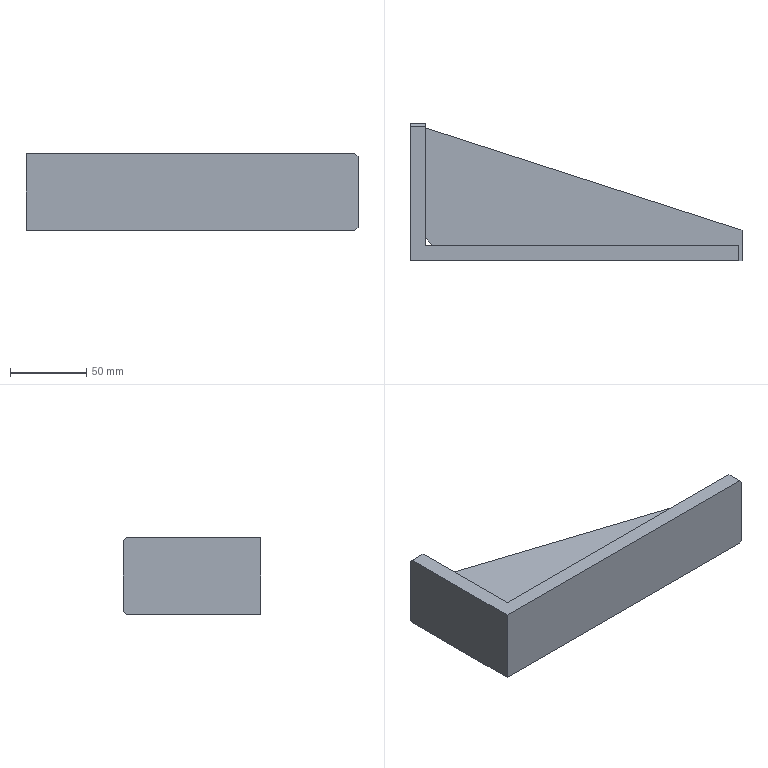Part | SolidWorks | features Chamfer 1, Extrusion 1, ICE 1 | 1 solid | 16 faces | box 217.5 x 90 x 50 mm | volume 220780 mm3 | plane 16
STEP:
#1=CARTESIAN_POINT('',(0.,88.,25.));
#2=VERTEX_POINT('',#1);
#3=CARTESIAN_POINT('',(0.,0.,25.));
#4=VERTEX_POINT('',#3);
#5=CARTESIAN_POINT('',(0.,90.,25.));
#6=DIRECTION('',(0.,-1.,0.));
#7=VECTOR('',#6,1000.);
#8=LINE('',#5,#7);
#9=EDGE_CURVE('',#2,#4,#8,.T.);
#10=ORIENTED_EDGE('',*,*,#9,.F.);
#11=CARTESIAN_POINT('',(0.,90.,23.));
#12=VERTEX_POINT('',#11);
#13=CARTESIAN_POINT('',(0.,88.,25.));
#14=DIRECTION('',(0.,0.7071,-0.7071));
#15=VECTOR('',#14,1000.);
#16=LINE('',#13,#15);
#17=EDGE_CURVE('',#2,#12,#16,.T.);
#18=ORIENTED_EDGE('',*,*,#17,.T.);
#19=CARTESIAN_POINT('',(0.,90.,-23.));
#20=VERTEX_POINT('',#19);
#21=CARTESIAN_POINT('',(0.,90.,25.));
#22=DIRECTION('',(0.,0.,-1.));
#23=VECTOR('',#22,1000.);
#24=LINE('',#21,#23);
#25=EDGE_CURVE('',#12,#20,#24,.T.);
#26=ORIENTED_EDGE('',*,*,#25,.T.);
#27=CARTESIAN_POINT('',(0.,88.,-25.));
#28=VERTEX_POINT('',#27);
#29=CARTESIAN_POINT('',(0.,90.,-23.));
#30=DIRECTION('',(0.,-0.7071,-0.7071));
#31=VECTOR('',#30,1000.);
#32=LINE('',#29,#31);
#33=EDGE_CURVE('',#20,#28,#32,.T.);
#34=ORIENTED_EDGE('',*,*,#33,.T.);
#35=CARTESIAN_POINT('',(0.,0.,-25.));
#36=VERTEX_POINT('',#35);
#37=CARTESIAN_POINT('',(0.,90.,-25.));
#38=DIRECTION('',(0.,-1.,0.));
#39=VECTOR('',#38,1000.);
#40=LINE('',#37,#39);
#41=EDGE_CURVE('',#28,#36,#40,.T.);
#42=ORIENTED_EDGE('',*,*,#41,.T.);
#43=CARTESIAN_POINT('',(0.,0.,25.));
#44=DIRECTION('',(0.,0.,-1.));
#45=VECTOR('',#44,1000.);
#46=LINE('',#43,#45);
#47=EDGE_CURVE('',#4,#36,#46,.T.);
#48=ORIENTED_EDGE('',*,*,#47,.F.);
#49=EDGE_LOOP('',(#10,#18,#26,#34,#42,#48));
#50=FACE_OUTER_BOUND('',#49,.T.);
#51=CARTESIAN_POINT('',(0.,90.,25.));
#52=DIRECTION('',(1.,0.,0.));
#53=DIRECTION('',(0.,1.,0.));
#54=AXIS2_PLACEMENT_3D('',#51,#52,#53);
#55=PLANE('',#54);
#56=ADVANCED_FACE('',(#50),#55,.F.);
#57=CARTESIAN_POINT('',(215.5,0.,-25.));
#58=VERTEX_POINT('',#57);
#59=CARTESIAN_POINT('',(0.,0.,-25.));
#60=DIRECTION('',(1.,0.,0.));
#61=VECTOR('',#60,1000.);
#62=LINE('',#59,#61);
#63=EDGE_CURVE('',#36,#58,#62,.T.);
#64=ORIENTED_EDGE('',*,*,#63,.T.);
#65=CARTESIAN_POINT('',(217.5,0.,-23.));
#66=VERTEX_POINT('',#65);
#67=CARTESIAN_POINT('',(217.5,0.,-23.));
#68=DIRECTION('',(0.7071,0.,0.7071));
#69=VECTOR('',#68,1000.);
#70=LINE('',#67,#69);
#71=EDGE_CURVE('',#58,#66,#70,.T.);
#72=ORIENTED_EDGE('',*,*,#71,.T.);
#73=CARTESIAN_POINT('',(217.5,0.,23.));
#74=VERTEX_POINT('',#73);
#75=CARTESIAN_POINT('',(217.5,0.,25.));
#76=DIRECTION('',(0.,0.,-1.));
#77=VECTOR('',#76,1000.);
#78=LINE('',#75,#77);
#79=EDGE_CURVE('',#74,#66,#78,.T.);
#80=ORIENTED_EDGE('',*,*,#79,.F.);
#81=CARTESIAN_POINT('',(215.5,0.,25.));
#82=VERTEX_POINT('',#81);
#83=CARTESIAN_POINT('',(215.5,0.,25.));
#84=DIRECTION('',(-0.7071,0.,0.7071));
#85=VECTOR('',#84,1000.);
#86=LINE('',#83,#85);
#87=EDGE_CURVE('',#74,#82,#86,.T.);
#88=ORIENTED_EDGE('',*,*,#87,.T.);
#89=CARTESIAN_POINT('',(0.,0.,25.));
#90=DIRECTION('',(1.,0.,0.));
#91=VECTOR('',#90,1000.);
#92=LINE('',#89,#91);
#93=EDGE_CURVE('',#4,#82,#92,.T.);
#94=ORIENTED_EDGE('',*,*,#93,.F.);
#95=ORIENTED_EDGE('',*,*,#47,.T.);
#96=EDGE_LOOP('',(#64,#72,#80,#88,#94,#95));
#97=FACE_OUTER_BOUND('',#96,.T.);
#98=CARTESIAN_POINT('',(0.,0.,25.));
#99=DIRECTION('',(0.,1.,0.));
#100=DIRECTION('',(0.,0.,1.));
#101=AXIS2_PLACEMENT_3D('',#98,#99,#100);
#102=PLANE('',#101);
#103=ADVANCED_FACE('',(#97),#102,.F.);
#104=ORIENTED_EDGE('',*,*,#79,.T.);
#105=CARTESIAN_POINT('',(217.5,10.,-23.));
#106=VERTEX_POINT('',#105);
#107=CARTESIAN_POINT('',(217.5,0.,-23.));
#108=DIRECTION('',(0.,1.,0.));
#109=VECTOR('',#108,1000.);
#110=LINE('',#107,#109);
#111=EDGE_CURVE('',#66,#106,#110,.T.);
#112=ORIENTED_EDGE('',*,*,#111,.T.);
#113=CARTESIAN_POINT('',(217.5,10.,-4.));
#114=VERTEX_POINT('',#113);
#115=CARTESIAN_POINT('',(217.5,10.,25.));
#116=DIRECTION('',(0.,0.,-1.));
#117=VECTOR('',#116,1000.);
#118=LINE('',#115,#117);
#119=EDGE_CURVE('',#114,#106,#118,.T.);
#120=ORIENTED_EDGE('',*,*,#119,.F.);
#121=CARTESIAN_POINT('',(217.5,20.,-4.));
#122=VERTEX_POINT('',#121);
#123=CARTESIAN_POINT('',(217.5,20.,-4.));
#124=DIRECTION('',(0.,1.,0.));
#125=VECTOR('',#124,1000.);
#126=LINE('',#123,#125);
#127=EDGE_CURVE('',#114,#122,#126,.T.);
#128=ORIENTED_EDGE('',*,*,#127,.T.);
#129=CARTESIAN_POINT('',(217.5,20.,4.));
#130=VERTEX_POINT('',#129);
#131=CARTESIAN_POINT('',(217.5,20.,4.));
#132=DIRECTION('',(0.,0.,-1.));
#133=VECTOR('',#132,1000.);
#134=LINE('',#131,#133);
#135=EDGE_CURVE('',#130,#122,#134,.T.);
#136=ORIENTED_EDGE('',*,*,#135,.F.);
#137=CARTESIAN_POINT('',(217.5,10.,4.));
#138=VERTEX_POINT('',#137);
#139=CARTESIAN_POINT('',(217.5,20.,4.));
#140=DIRECTION('',(0.,1.,0.));
#141=VECTOR('',#140,1000.);
#142=LINE('',#139,#141);
#143=EDGE_CURVE('',#138,#130,#142,.T.);
#144=ORIENTED_EDGE('',*,*,#143,.F.);
#145=CARTESIAN_POINT('',(217.5,10.,23.));
#146=VERTEX_POINT('',#145);
#147=CARTESIAN_POINT('',(217.5,10.,25.));
#148=DIRECTION('',(0.,0.,-1.));
#149=VECTOR('',#148,1000.);
#150=LINE('',#147,#149);
#151=EDGE_CURVE('',#146,#138,#150,.T.);
#152=ORIENTED_EDGE('',*,*,#151,.F.);
#153=CARTESIAN_POINT('',(217.5,0.,23.));
#154=DIRECTION('',(0.,-1.,0.));
#155=VECTOR('',#154,1000.);
#156=LINE('',#153,#155);
#157=EDGE_CURVE('',#146,#74,#156,.T.);
#158=ORIENTED_EDGE('',*,*,#157,.T.);
#159=EDGE_LOOP('',(#104,#112,#120,#128,#136,#144,#152,#158));
#160=FACE_OUTER_BOUND('',#159,.T.);
#161=CARTESIAN_POINT('',(217.5,0.,25.));
#162=DIRECTION('',(-1.,0.,0.));
#163=DIRECTION('',(0.,0.,1.));
#164=AXIS2_PLACEMENT_3D('',#161,#162,#163);
#165=PLANE('',#164);
#166=ADVANCED_FACE('',(#160),#165,.F.);
#167=ORIENTED_EDGE('',*,*,#119,.T.);
#168=CARTESIAN_POINT('',(215.5,10.,-25.));
#169=VERTEX_POINT('',#168);
#170=CARTESIAN_POINT('',(217.5,10.,-23.));
#171=DIRECTION('',(-0.7071,0.,-0.7071));
#172=VECTOR('',#171,1000.);
#173=LINE('',#170,#172);
#174=EDGE_CURVE('',#106,#169,#173,.T.);
#175=ORIENTED_EDGE('',*,*,#174,.T.);
#176=CARTESIAN_POINT('',(10.,10.,-25.));
#177=VERTEX_POINT('',#176);
#178=CARTESIAN_POINT('',(217.5,10.,-25.));
#179=DIRECTION('',(-1.,0.,0.));
#180=VECTOR('',#179,1000.);
#181=LINE('',#178,#180);
#182=EDGE_CURVE('',#169,#177,#181,.T.);
#183=ORIENTED_EDGE('',*,*,#182,.T.);
#184=CARTESIAN_POINT('',(10.,10.,25.));
#185=VERTEX_POINT('',#184);
#186=CARTESIAN_POINT('',(10.,10.,25.));
#187=DIRECTION('',(0.,0.,-1.));
#188=VECTOR('',#187,1000.);
#189=LINE('',#186,#188);
#190=EDGE_CURVE('',#185,#177,#189,.T.);
#191=ORIENTED_EDGE('',*,*,#190,.F.);
#192=CARTESIAN_POINT('',(215.5,10.,25.));
#193=VERTEX_POINT('',#192);
#194=CARTESIAN_POINT('',(217.5,10.,25.));
#195=DIRECTION('',(-1.,0.,0.));
#196=VECTOR('',#195,1000.);
#197=LINE('',#194,#196);
#198=EDGE_CURVE('',#193,#185,#197,.T.);
#199=ORIENTED_EDGE('',*,*,#198,.F.);
#200=CARTESIAN_POINT('',(215.5,10.,25.));
#201=DIRECTION('',(0.7071,0.,-0.7071));
#202=VECTOR('',#201,1000.);
#203=LINE('',#200,#202);
#204=EDGE_CURVE('',#193,#146,#203,.T.);
#205=ORIENTED_EDGE('',*,*,#204,.T.);
#206=ORIENTED_EDGE('',*,*,#151,.T.);
#207=CARTESIAN_POINT('',(15.,10.,4.));
#208=VERTEX_POINT('',#207);
#209=CARTESIAN_POINT('',(217.5,10.,4.));
#210=DIRECTION('',(1.,0.,0.));
#211=VECTOR('',#210,1000.);
#212=LINE('',#209,#211);
#213=EDGE_CURVE('',#208,#138,#212,.T.);
#214=ORIENTED_EDGE('',*,*,#213,.F.);
#215=CARTESIAN_POINT('',(15.,10.,-4.));
#216=VERTEX_POINT('',#215);
#217=CARTESIAN_POINT('',(15.,10.,4.));
#218=DIRECTION('',(0.,0.,-1.));
#219=VECTOR('',#218,1000.);
#220=LINE('',#217,#219);
#221=EDGE_CURVE('',#208,#216,#220,.T.);
#222=ORIENTED_EDGE('',*,*,#221,.T.);
#223=CARTESIAN_POINT('',(217.5,10.,-4.));
#224=DIRECTION('',(1.,0.,0.));
#225=VECTOR('',#224,1000.);
#226=LINE('',#223,#225);
#227=EDGE_CURVE('',#216,#114,#226,.T.);
#228=ORIENTED_EDGE('',*,*,#227,.T.);
#229=EDGE_LOOP('',(#167,#175,#183,#191,#199,#205,#206,#214,#222,#228));
#230=FACE_OUTER_BOUND('',#229,.T.);
#231=CARTESIAN_POINT('',(217.5,10.,25.));
#232=DIRECTION('',(0.,-1.,0.));
#233=DIRECTION('',(1.,0.,0.));
#234=AXIS2_PLACEMENT_3D('',#231,#232,#233);
#235=PLANE('',#234);
#236=ADVANCED_FACE('',(#230),#235,.F.);
#237=CARTESIAN_POINT('',(10.,15.,4.));
#238=VERTEX_POINT('',#237);
#239=CARTESIAN_POINT('',(10.,15.,-4.));
#240=VERTEX_POINT('',#239);
#241=CARTESIAN_POINT('',(10.,15.,4.));
#242=DIRECTION('',(0.,0.,-1.));
#243=VECTOR('',#242,1000.);
#244=LINE('',#241,#243);
#245=EDGE_CURVE('',#238,#240,#244,.T.);
#246=ORIENTED_EDGE('',*,*,#245,.F.);
#247=CARTESIAN_POINT('',(10.,87.,4.));
#248=VERTEX_POINT('',#247);
#249=CARTESIAN_POINT('',(10.,15.,4.));
#250=DIRECTION('',(0.,-1.,0.));
#251=VECTOR('',#250,1000.);
#252=LINE('',#249,#251);
#253=EDGE_CURVE('',#248,#238,#252,.T.);
#254=ORIENTED_EDGE('',*,*,#253,.F.);
#255=CARTESIAN_POINT('',(10.,87.,-4.));
#256=VERTEX_POINT('',#255);
#257=CARTESIAN_POINT('',(10.,87.,4.));
#258=DIRECTION('',(0.,0.,-1.));
#259=VECTOR('',#258,1000.);
#260=LINE('',#257,#259);
#261=EDGE_CURVE('',#248,#256,#260,.T.);
#262=ORIENTED_EDGE('',*,*,#261,.T.);
#263=CARTESIAN_POINT('',(10.,15.,-4.));
#264=DIRECTION('',(0.,-1.,0.));
#265=VECTOR('',#264,1000.);
#266=LINE('',#263,#265);
#267=EDGE_CURVE('',#256,#240,#266,.T.);
#268=ORIENTED_EDGE('',*,*,#267,.T.);
#269=EDGE_LOOP('',(#246,#254,#262,#268));
#270=FACE_BOUND('',#269,.T.);
#271=CARTESIAN_POINT('',(10.,90.,23.));
#272=VERTEX_POINT('',#271);
#273=CARTESIAN_POINT('',(10.,90.,-23.));
#274=VERTEX_POINT('',#273);
#275=CARTESIAN_POINT('',(10.,90.,25.));
#276=DIRECTION('',(0.,0.,-1.));
#277=VECTOR('',#276,1000.);
#278=LINE('',#275,#277);
#279=EDGE_CURVE('',#272,#274,#278,.T.);
#280=ORIENTED_EDGE('',*,*,#279,.F.);
#281=CARTESIAN_POINT('',(10.,88.,25.));
#282=VERTEX_POINT('',#281);
#283=CARTESIAN_POINT('',(10.,88.,25.));
#284=DIRECTION('',(0.,-0.7071,0.7071));
#285=VECTOR('',#284,1000.);
#286=LINE('',#283,#285);
#287=EDGE_CURVE('',#272,#282,#286,.T.);
#288=ORIENTED_EDGE('',*,*,#287,.T.);
#289=CARTESIAN_POINT('',(10.,10.,25.));
#290=DIRECTION('',(0.,1.,0.));
#291=VECTOR('',#290,1000.);
#292=LINE('',#289,#291);
#293=EDGE_CURVE('',#185,#282,#292,.T.);
#294=ORIENTED_EDGE('',*,*,#293,.F.);
#295=ORIENTED_EDGE('',*,*,#190,.T.);
#296=CARTESIAN_POINT('',(10.,88.,-25.));
#297=VERTEX_POINT('',#296);
#298=CARTESIAN_POINT('',(10.,10.,-25.));
#299=DIRECTION('',(0.,1.,0.));
#300=VECTOR('',#299,1000.);
#301=LINE('',#298,#300);
#302=EDGE_CURVE('',#177,#297,#301,.T.);
#303=ORIENTED_EDGE('',*,*,#302,.T.);
#304=CARTESIAN_POINT('',(10.,90.,-23.));
#305=DIRECTION('',(0.,0.7071,0.7071));
#306=VECTOR('',#305,1000.);
#307=LINE('',#304,#306);
#308=EDGE_CURVE('',#297,#274,#307,.T.);
#309=ORIENTED_EDGE('',*,*,#308,.T.);
#310=EDGE_LOOP('',(#280,#288,#294,#295,#303,#309));
#311=FACE_OUTER_BOUND('',#310,.T.);
#312=CARTESIAN_POINT('',(10.,10.,25.));
#313=DIRECTION('',(-1.,0.,0.));
#314=DIRECTION('',(0.,-1.,0.));
#315=AXIS2_PLACEMENT_3D('',#312,#313,#314);
#316=PLANE('',#315);
#317=ADVANCED_FACE('',(#270,#311),#316,.F.);
#318=ORIENTED_EDGE('',*,*,#25,.F.);
#319=CARTESIAN_POINT('',(10.,90.,23.));
#320=DIRECTION('',(1.,0.,0.));
#321=VECTOR('',#320,1000.);
#322=LINE('',#319,#321);
#323=EDGE_CURVE('',#12,#272,#322,.T.);
#324=ORIENTED_EDGE('',*,*,#323,.T.);
#325=ORIENTED_EDGE('',*,*,#279,.T.);
#326=CARTESIAN_POINT('',(10.,90.,-23.));
#327=DIRECTION('',(-1.,0.,0.));
#328=VECTOR('',#327,1000.);
#329=LINE('',#326,#328);
#330=EDGE_CURVE('',#274,#20,#329,.T.);
#331=ORIENTED_EDGE('',*,*,#330,.T.);
#332=EDGE_LOOP('',(#318,#324,#325,#331));
#333=FACE_OUTER_BOUND('',#332,.T.);
#334=CARTESIAN_POINT('',(10.,90.,25.));
#335=DIRECTION('',(0.,-1.,0.));
#336=DIRECTION('',(0.,0.,-1.));
#337=AXIS2_PLACEMENT_3D('',#334,#335,#336);
#338=PLANE('',#337);
#339=ADVANCED_FACE('',(#333),#338,.F.);
#340=ORIENTED_EDGE('',*,*,#93,.T.);
#341=CARTESIAN_POINT('',(215.5,10.,25.));
#342=DIRECTION('',(0.,1.,0.));
#343=VECTOR('',#342,1000.);
#344=LINE('',#341,#343);
#345=EDGE_CURVE('',#82,#193,#344,.T.);
#346=ORIENTED_EDGE('',*,*,#345,.T.);
#347=ORIENTED_EDGE('',*,*,#198,.T.);
#348=ORIENTED_EDGE('',*,*,#293,.T.);
#349=CARTESIAN_POINT('',(0.,88.,25.));
#350=DIRECTION('',(-1.,0.,0.));
#351=VECTOR('',#350,1000.);
#352=LINE('',#349,#351);
#353=EDGE_CURVE('',#282,#2,#352,.T.);
#354=ORIENTED_EDGE('',*,*,#353,.T.);
#355=ORIENTED_EDGE('',*,*,#9,.T.);
#356=EDGE_LOOP('',(#340,#346,#347,#348,#354,#355));
#357=FACE_OUTER_BOUND('',#356,.T.);
#358=CARTESIAN_POINT('',(0.,0.,25.));
#359=DIRECTION('',(0.,0.,1.));
#360=DIRECTION('',(1.,0.,0.));
#361=AXIS2_PLACEMENT_3D('',#358,#359,#360);
#362=PLANE('',#361);
#363=ADVANCED_FACE('',(#357),#362,.T.);
#364=ORIENTED_EDGE('',*,*,#182,.F.);
#365=CARTESIAN_POINT('',(215.5,0.,-25.));
#366=DIRECTION('',(0.,-1.,0.));
#367=VECTOR('',#366,1000.);
#368=LINE('',#365,#367);
#369=EDGE_CURVE('',#169,#58,#368,.T.);
#370=ORIENTED_EDGE('',*,*,#369,.T.);
#371=ORIENTED_EDGE('',*,*,#63,.F.);
#372=ORIENTED_EDGE('',*,*,#41,.F.);
#373=CARTESIAN_POINT('',(0.,88.,-25.));
#374=DIRECTION('',(1.,0.,0.));
#375=VECTOR('',#374,1000.);
#376=LINE('',#373,#375);
#377=EDGE_CURVE('',#28,#297,#376,.T.);
#378=ORIENTED_EDGE('',*,*,#377,.T.);
#379=ORIENTED_EDGE('',*,*,#302,.F.);
#380=EDGE_LOOP('',(#364,#370,#371,#372,#378,#379));
#381=FACE_OUTER_BOUND('',#380,.T.);
#382=CARTESIAN_POINT('',(0.,0.,-25.));
#383=DIRECTION('',(0.,0.,1.));
#384=DIRECTION('',(1.,0.,0.));
#385=AXIS2_PLACEMENT_3D('',#382,#383,#384);
#386=PLANE('',#385);
#387=ADVANCED_FACE('',(#381),#386,.F.);
#388=CARTESIAN_POINT('',(15.,10.,-4.));
#389=DIRECTION('',(0.7071,-0.7071,0.));
#390=VECTOR('',#389,1000.);
#391=LINE('',#388,#390);
#392=EDGE_CURVE('',#240,#216,#391,.T.);
#393=ORIENTED_EDGE('',*,*,#392,.T.);
#394=ORIENTED_EDGE('',*,*,#221,.F.);
#395=CARTESIAN_POINT('',(15.,10.,4.));
#396=DIRECTION('',(0.7071,-0.7071,0.));
#397=VECTOR('',#396,1000.);
#398=LINE('',#395,#397);
#399=EDGE_CURVE('',#238,#208,#398,.T.);
#400=ORIENTED_EDGE('',*,*,#399,.F.);
#401=ORIENTED_EDGE('',*,*,#245,.T.);
#402=EDGE_LOOP('',(#393,#394,#400,#401));
#403=FACE_OUTER_BOUND('',#402,.T.);
#404=CARTESIAN_POINT('',(15.,10.,4.));
#405=DIRECTION('',(0.7071,0.7071,0.));
#406=DIRECTION('',(-0.7071,0.7071,0.));
#407=AXIS2_PLACEMENT_3D('',#404,#405,#406);
#408=PLANE('',#407);
#409=ADVANCED_FACE('',(#403),#408,.F.);
#410=CARTESIAN_POINT('',(10.,87.,-4.));
#411=DIRECTION('',(-0.9516,0.3073,0.));
#412=VECTOR('',#411,1000.);
#413=LINE('',#410,#412);
#414=EDGE_CURVE('',#122,#256,#413,.T.);
#415=ORIENTED_EDGE('',*,*,#414,.T.);
#416=ORIENTED_EDGE('',*,*,#261,.F.);
#417=CARTESIAN_POINT('',(10.,87.,4.));
#418=DIRECTION('',(-0.9516,0.3073,0.));
#419=VECTOR('',#418,1000.);
#420=LINE('',#417,#419);
#421=EDGE_CURVE('',#130,#248,#420,.T.);
#422=ORIENTED_EDGE('',*,*,#421,.F.);
#423=ORIENTED_EDGE('',*,*,#135,.T.);
#424=EDGE_LOOP('',(#415,#416,#422,#423));
#425=FACE_OUTER_BOUND('',#424,.T.);
#426=CARTESIAN_POINT('',(10.,87.,4.));
#427=DIRECTION('',(-0.3073,-0.9516,0.));
#428=DIRECTION('',(0.9516,-0.3073,0.));
#429=AXIS2_PLACEMENT_3D('',#426,#427,#428);
#430=PLANE('',#429);
#431=ADVANCED_FACE('',(#425),#430,.F.);
#432=ORIENTED_EDGE('',*,*,#253,.T.);
#433=ORIENTED_EDGE('',*,*,#399,.T.);
#434=ORIENTED_EDGE('',*,*,#213,.T.);
#435=ORIENTED_EDGE('',*,*,#143,.T.);
#436=ORIENTED_EDGE('',*,*,#421,.T.);
#437=EDGE_LOOP('',(#432,#433,#434,#435,#436));
#438=FACE_OUTER_BOUND('',#437,.T.);
#439=CARTESIAN_POINT('',(0.,0.,4.));
#440=DIRECTION('',(0.,0.,1.));
#441=DIRECTION('',(1.,0.,0.));
#442=AXIS2_PLACEMENT_3D('',#439,#440,#441);
#443=PLANE('',#442);
#444=ADVANCED_FACE('',(#438),#443,.T.);
#445=ORIENTED_EDGE('',*,*,#267,.F.);
#446=ORIENTED_EDGE('',*,*,#414,.F.);
#447=ORIENTED_EDGE('',*,*,#127,.F.);
#448=ORIENTED_EDGE('',*,*,#227,.F.);
#449=ORIENTED_EDGE('',*,*,#392,.F.);
#450=EDGE_LOOP('',(#445,#446,#447,#448,#449));
#451=FACE_OUTER_BOUND('',#450,.T.);
#452=CARTESIAN_POINT('',(0.,0.,-4.));
#453=DIRECTION('',(0.,0.,1.));
#454=DIRECTION('',(1.,0.,0.));
#455=AXIS2_PLACEMENT_3D('',#452,#453,#454);
#456=PLANE('',#455);
#457=ADVANCED_FACE('',(#451),#456,.F.);
#458=ORIENTED_EDGE('',*,*,#71,.F.);
#459=ORIENTED_EDGE('',*,*,#369,.F.);
#460=ORIENTED_EDGE('',*,*,#174,.F.);
#461=ORIENTED_EDGE('',*,*,#111,.F.);
#462=EDGE_LOOP('',(#458,#459,#460,#461));
#463=FACE_OUTER_BOUND('',#462,.T.);
#464=CARTESIAN_POINT('',(217.5,0.,-23.));
#465=DIRECTION('',(-0.7071,0.,0.7071));
#466=DIRECTION('',(0.,1.,0.));
#467=AXIS2_PLACEMENT_3D('',#464,#465,#466);
#468=PLANE('',#467);
#469=ADVANCED_FACE('',(#463),#468,.F.);
#470=ORIENTED_EDGE('',*,*,#87,.F.);
#471=ORIENTED_EDGE('',*,*,#157,.F.);
#472=ORIENTED_EDGE('',*,*,#204,.F.);
#473=ORIENTED_EDGE('',*,*,#345,.F.);
#474=EDGE_LOOP('',(#470,#471,#472,#473));
#475=FACE_OUTER_BOUND('',#474,.T.);
#476=CARTESIAN_POINT('',(215.5,0.,25.));
#477=DIRECTION('',(0.7071,0.,0.7071));
#478=DIRECTION('',(0.,-1.,0.));
#479=AXIS2_PLACEMENT_3D('',#476,#477,#478);
#480=PLANE('',#479);
#481=ADVANCED_FACE('',(#475),#480,.T.);
#482=ORIENTED_EDGE('',*,*,#287,.F.);
#483=ORIENTED_EDGE('',*,*,#323,.F.);
#484=ORIENTED_EDGE('',*,*,#17,.F.);
#485=ORIENTED_EDGE('',*,*,#353,.F.);
#486=EDGE_LOOP('',(#482,#483,#484,#485));
#487=FACE_OUTER_BOUND('',#486,.T.);
#488=CARTESIAN_POINT('',(0.,88.,25.));
#489=DIRECTION('',(0.,0.7071,0.7071));
#490=DIRECTION('',(1.,0.,0.));
#491=AXIS2_PLACEMENT_3D('',#488,#489,#490);
#492=PLANE('',#491);
#493=ADVANCED_FACE('',(#487),#492,.T.);
#494=ORIENTED_EDGE('',*,*,#308,.F.);
#495=ORIENTED_EDGE('',*,*,#377,.F.);
#496=ORIENTED_EDGE('',*,*,#33,.F.);
#497=ORIENTED_EDGE('',*,*,#330,.F.);
#498=EDGE_LOOP('',(#494,#495,#496,#497));
#499=FACE_OUTER_BOUND('',#498,.T.);
#500=CARTESIAN_POINT('',(10.,90.,-23.));
#501=DIRECTION('',(0.,-0.7071,0.7071));
#502=DIRECTION('',(-1.,0.,0.));
#503=AXIS2_PLACEMENT_3D('',#500,#501,#502);
#504=PLANE('',#503);
#505=ADVANCED_FACE('',(#499),#504,.F.);
#506=CLOSED_SHELL('',(#56,#103,#166,#236,#317,#339,#363,#387,#409,#431,#444,#457,#469,#481,#493,#505));
#507=MANIFOLD_SOLID_BREP('',#506);
#508=CARTESIAN_POINT('',(0.,0.,0.));
#509=DIRECTION('',(0.,0.,1.));
#510=DIRECTION('',(1.,0.,0.));
#511=AXIS2_PLACEMENT_3D('',#508,#509,#510);
#512=(LENGTH_UNIT()NAMED_UNIT(*)SI_UNIT(.MILLI.,.METRE.));
#513=UNCERTAINTY_MEASURE_WITH_UNIT(LENGTH_MEASURE(0.00001),#512,'','');
#514=(NAMED_UNIT(*)PLANE_ANGLE_UNIT()SI_UNIT($,.RADIAN.));
#515=(NAMED_UNIT(*)SI_UNIT($,.STERADIAN.)SOLID_ANGLE_UNIT());
#516=(GEOMETRIC_REPRESENTATION_CONTEXT(3)GLOBAL_UNCERTAINTY_ASSIGNED_CONTEXT((#513))GLOBAL_UNIT_ASSIGNED_CONTEXT((#512,#514,#515))REPRESENTATION_CONTEXT('',''));
#517=ADVANCED_BREP_SHAPE_REPRESENTATION('',(#507,#511),#516);